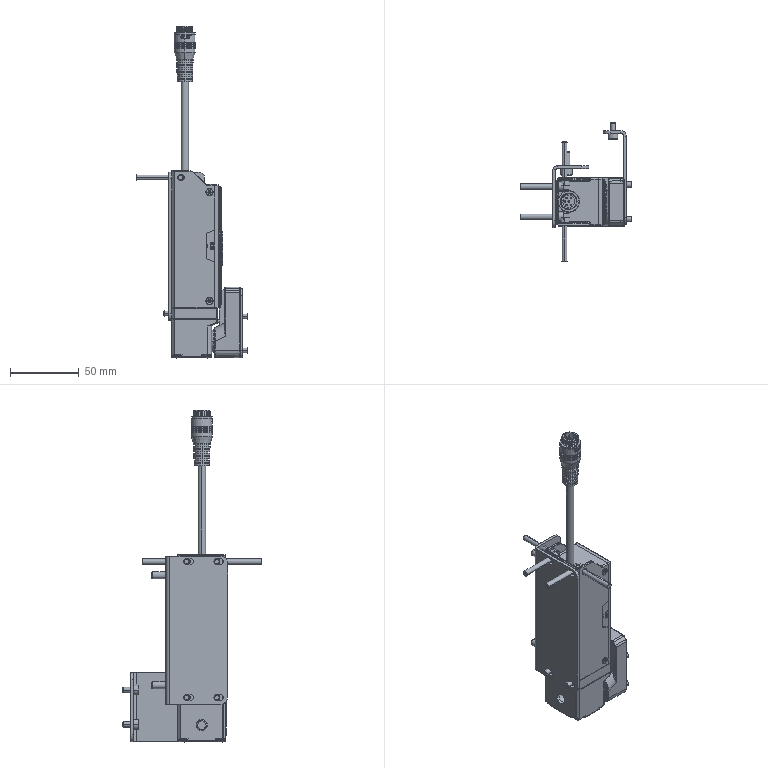Part | SolidWorks | 21 solids | 4346 faces | volume 117384 mm3 | plane 1921 | cylinder 1166 | cone 711 | spline 279 | torus 223 | sphere 46 | commonest cylinder face diameters 2.5 x178 1 x161 2 x86 0.4 x84 4.5 x53 5 x46